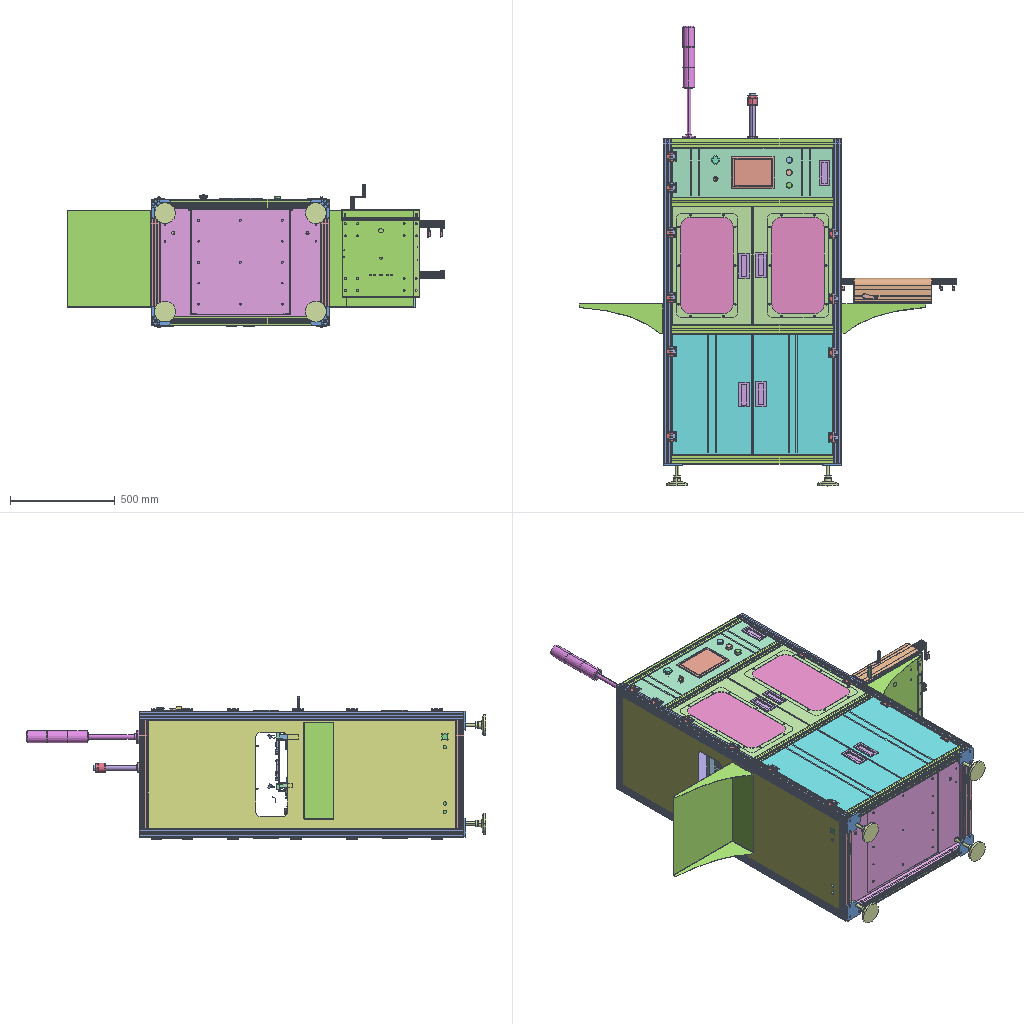Assembly | STEP file | 123 different items | 361 placed | box 1801 x 2194 x 686 mm
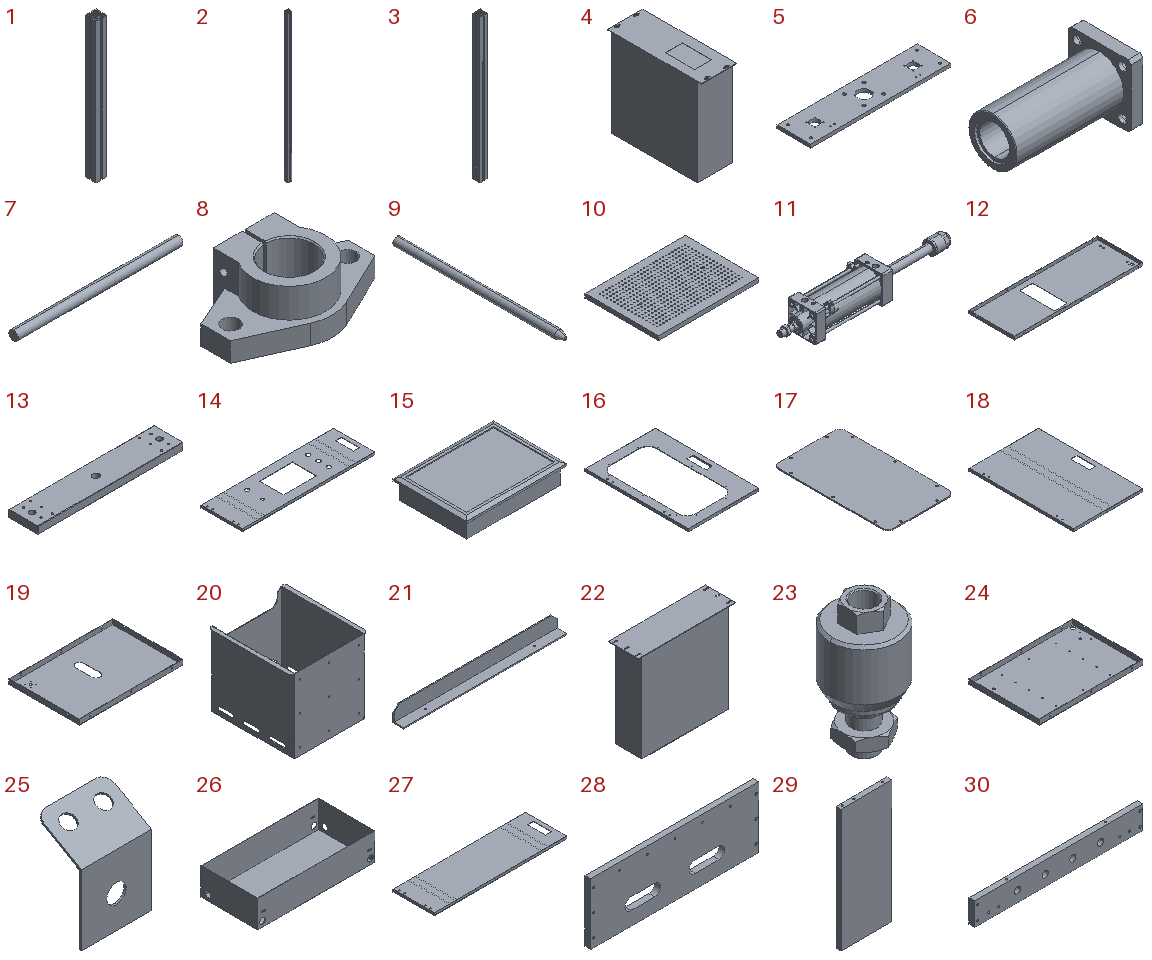Parts list (item | name | quantity | parent item | size | volume):
1 | Frame aluminum channel 3 | x9 | in FCT online single-layer test machine | 40 x 40 x 520 mm | 336590 mm3
2 | ICT frame aluminum channel 1 | x4 | in FCT online single-layer test machine | 40 x 40 x 1550 mm | 1003296 mm3
3 | Frame aluminum channel 2 | x8 | in FCT online single-layer test machine | 40 x 40 x 770 mm | 498412 mm3
4 | Industrial PC | x1 | in FCT online single-layer test machine | 180 x 480 x 450 mm | 35646453 mm3
5 | Hold-down fixture fixing plate | x1 | in FCT online single-layer test machine | 500 x 120 x 12 mm | 670055 mm3
6 | LMK20LUU  | x2 | in FCT online single-layer test machine | 80 x 42 x 42 mm | 44458 mm3
7 | Hold-down sync guide rod | x2 | in FCT online single-layer test machine | 350 x 20 x 20 mm | 109206 mm3
8 | SHF20 | x2 | in FCT online single-layer test machine | 60 x 36.276 x 20 mm | 15283 mm3
9 | Press rod | x4 | in FCT online single-layer test machine | 6 x 125 x 6 mm | 3458 mm3
10 | FCT press block | x1 | in FCT online single-layer test machine | 480 x 350 x 20 mm | 3170211 mm3
11 | SCJ_80x150_20_S_A_2_0020_ retract | x1 | in FCT online single-layer test machine | - | -
12 | ICT side seal plate | x2 | in FCT online single-layer test machine | 1468 x 518 x 38 mm | 1263222 mm3
13 | Hold-down fixture fixing plate | x1 | in FCT online single-layer test machine | 400 x 80 x 20 mm | 625122 mm3
14 | Front upper door | x1 | in FCT online single-layer test machine | 767 x 237 x 15 mm | 445389 mm3
15 | Xinje TH765 touch screen | x1 | in FCT online single-layer test machine | 204 x 150.5 x 44 mm | 1119032 mm3
16 | Middle door | x4 | in Door | 382.5 x 565 x 15 mm | 308904 mm3
17 | PVC sealing plate | x4 | in Door | 290 x 500 x 5 mm | 719804 mm3
18 | Bottom door | x4 | in FCT online single-layer test machine | 382.5 x 579 x 15 mm | 596109 mm3
19 | Top seal plate | x1 | in FCT online single-layer test machine | 768 x 518 x 38 mm | 719559 mm3
20 | Electrical cabinet box | x1 | in FCT online single-layer test machine | 520 x 560 x 500 mm | 2941429 mm3
21 | Electrical cabinet partition strip | x1 | in FCT online single-layer test machine | 450 x 30 x 40 mm | 89657 mm3
22 | FCT electrical control box | x1 | in FCT online single-layer test machine | 520 x 160 x 483 mm | 872599 mm3
23 | F-M20150F floating joint_HI | x1 | in FCT online single-layer test machine | 53 x 53 x 102 mm | 127493 mm3
24 | Bottom seal plate | x1 | in FCT online single-layer test machine | 768 x 518 x 38 mm | 730452 mm3
25 | Fiber fixing plate | x2 | in FCT online single-layer test machine, Conveyor test structure assembly | 20 x 13.29 x 27.5 mm | 382.645 mm3
26 | ICT test machine electrical box | x1 | in FCT online single-layer test machine | 515 x 250 x 120 mm | 459009 mm3
27 | Rear upper door | x1 | in FCT online single-layer test machine | 767 x 237 x 15 mm | 502024 mm3
28 | Rear side plate | x1 | in Test assembly | 425 x 15 x 155 mm | 907498 mm3
29 | Left-right side plate | x1 | in Test assembly | 155 x 15 x 375 mm | 868144 mm3
30 | Front side plate B | x1 | in Test assembly | 425 x 15 x 58 mm | 353146 mm3
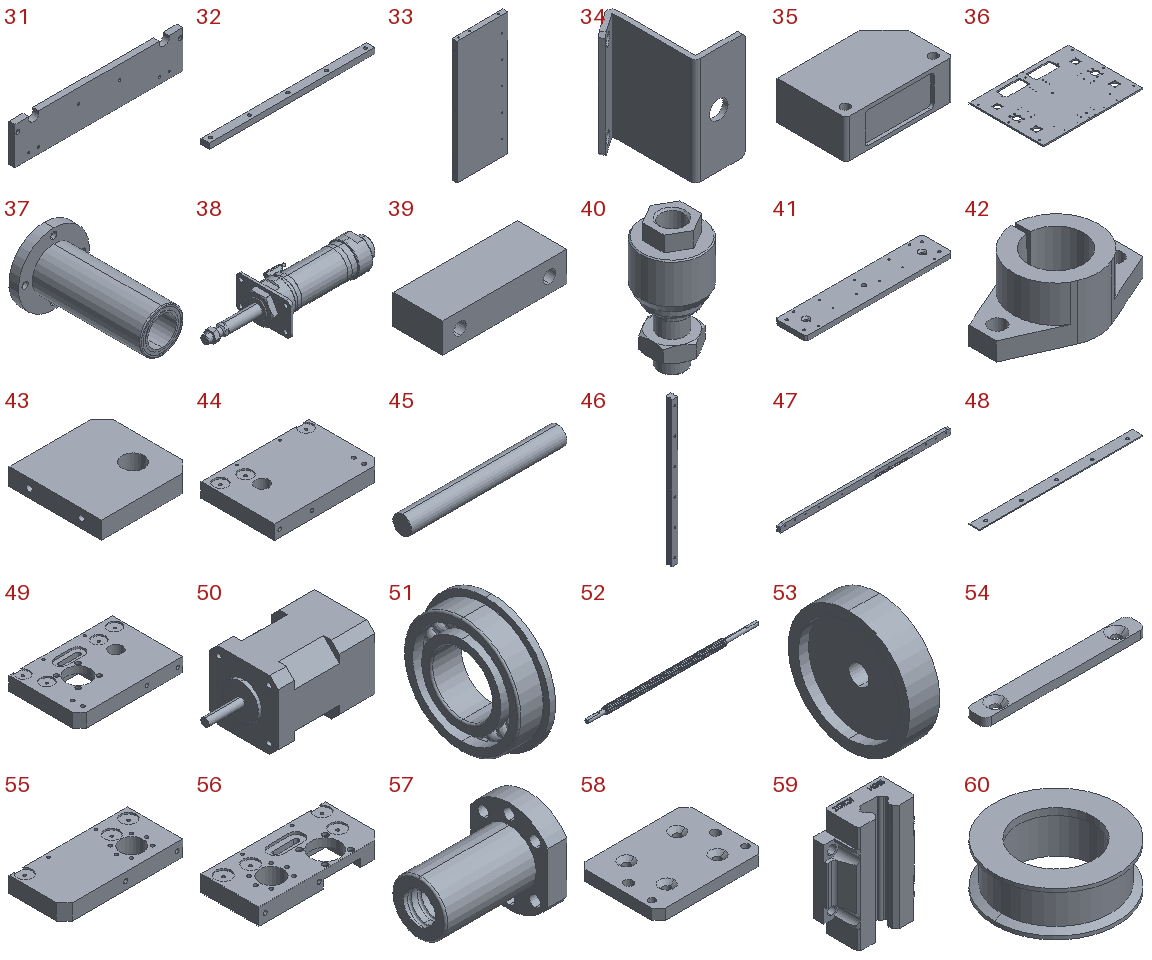31 | Front side plate A | x1 | in Test assembly | 425 x 15 x 95 mm | 590562 mm3
32 | Glass fixing plate | x4 | in Test assembly | 300 x 15 x 10 mm | 42251 mm3
33 | Left-right side plate A | x1 | in Test assembly | 155 x 15 x 375 mm | 868153 mm3
34 | Photoelectric switch mounting plate | x2 | in Photoelectric switch assembly | 22.414 x 26.5 x 32 mm | 2228 mm3
35 | CX421 | x2 | in Photoelectric switch assembly | 31.036 x 20.036 x 11.2 mm | 6433 mm3
36 | Platform plate | x1 | in Test mechanism assembly | 765 x 570 x 10 mm | 3949080 mm3
37 | LMF30LUU | x4 | in Test mechanism assembly | 74 x 123 x 74 mm | 132378 mm3
38 | MAL40x50-S-CM-FA-M-2 synchronous | x2 | in Test mechanism assembly | - | -
39 | Cylinder pad plate | x4 | in Test mechanism assembly | 50 x 20 x 12 mm | 11215 mm3
40 | F-M12125F floating joint | x2 | in Test mechanism assembly | 28 x 28 x 58 mm | 19289 mm3
41 | Width adjustment base | x2 | in Rail assembly | 380 x 80 x 12 mm | 356572 mm3
42 | SHF30 | x4 | in Rail assembly | 80 x 48 x 30 mm | 36862 mm3
43 | Lead screw rear fixing plate | x2 | in Rail assembly | 80 x 80 x 15 mm | 89638 mm3
44 | Front rail (left) | x1 | in Rail assembly | 150 x 102 x 20 mm | 295247 mm3
45 | Rail sync guide rod | x4 | in Rail assembly | 250 x 30 x 30 mm | 175961 mm3
46 | 15 guide rail | x2 | in Rail assembly | 15 x 15 x 330 mm | 60891 mm3
47 | Rail | x2 | in Rail assembly, Rear rail assembly | 840 x 15 x 30 mm | 357627 mm3
48 | Belt bracket plate | x2 | in Rail assembly, Rear rail assembly | 530 x 34 x 3 mm | 53588 mm3
49 | Front rail (right) | x1 | in Rail assembly | 150 x 102 x 20 mm | 257499 mm3
50 | Stepper motor CT2H420068-011 | x2 | in Rail assembly, Rear rail assembly | 84 x 42.3 x 42.3 mm | 101112 mm3
51 | miniature radial ball bearings gb_Rolling bearings FF61800  GB 7218-1995 | x4 | in Rail assembly | 5 x 21 x 21 mm | 818.239 mm3
52 | 1605 ball screw | x2 | in Rail assembly | 440 x 16 x 16 mm | 67458 mm3
53 | Handle | x2 | in Rail assembly | 25 x 60 x 60 mm | 35825 mm3
54 | Belt support strip | x4 | in Rail assembly, Rear rail assembly | 80 x 10 x 4 mm | 2948 mm3
55 | Rear rail (left) | x1 | in Rear rail assembly | 150 x 70 x 20 mm | 191088 mm3
56 | Rear rail (right) | x1 | in Rear rail assembly | 150 x 70 x 20 mm | 154483 mm3
57 | SHF1605 nut | x2 | in Rear rail assembly | 57 x 40 x 48 mm | 31691 mm3
58 | Slider connection plate | x2 | in Rear rail assembly | 80 x 60 x 8 mm | 35674 mm3
59 | HGW15CC slider | x2 | in Rear rail assembly | 47 x 19.7 x 61.7 mm | 35571 mm3
60 | 602-08-0005 | x16 | in 604 bearing assembly | 18 x 18 x 6.5 mm | 669.421 mm3
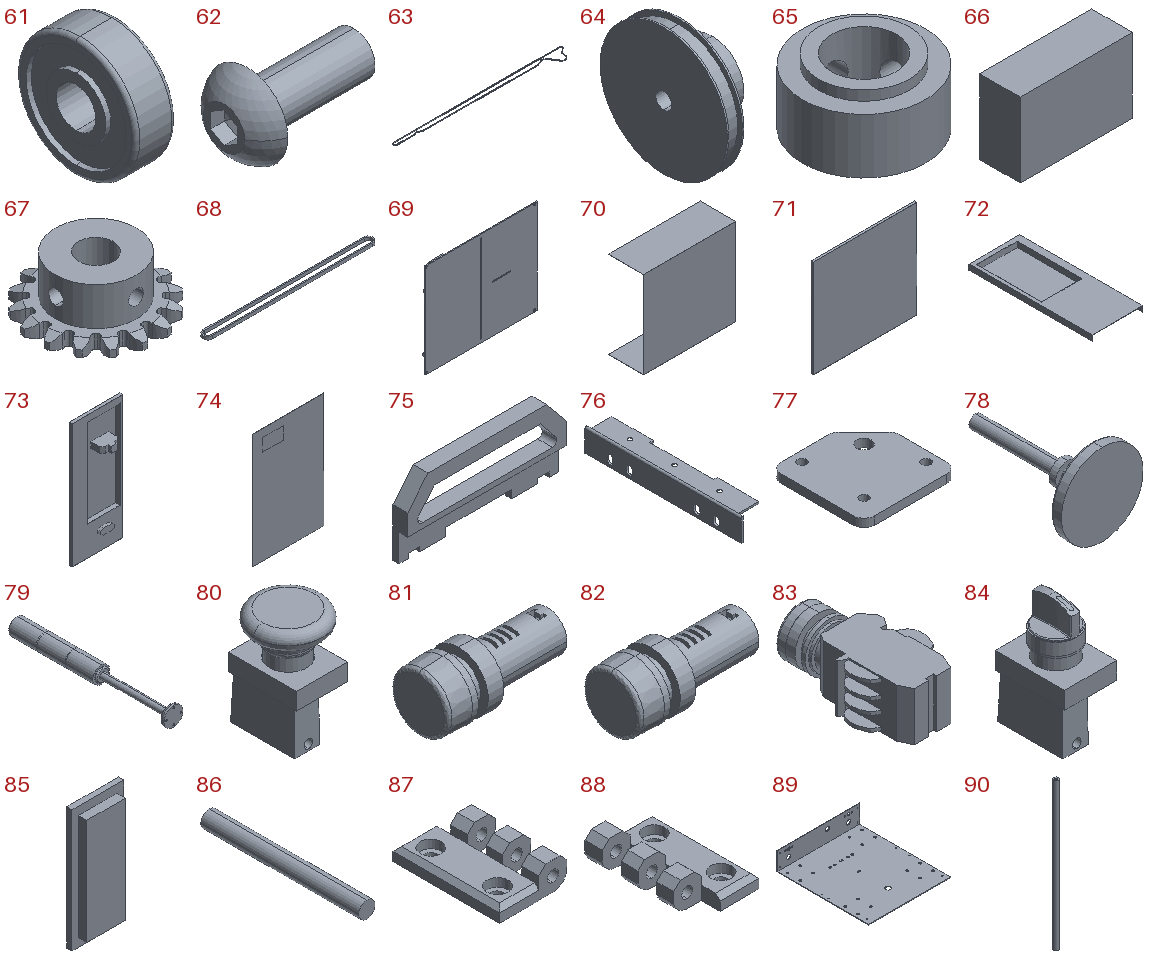61 | 604 bearing | x16 | in 604 bearing assembly | 4 x 12 x 12 mm | 349.308 mm3
62 | hexagon socket button head screws gb_GB_SOCKET_TYPE7 M4X10-N | x16 | in 604 bearing assembly | 12.2 x 7.6 x 7.6 mm | 185.741 mm3
63 | Belt | x2 | in Rear rail assembly, Rail assembly | 833 x 69.5 x 4 mm | 6996 mm3
64 | Belt drive pulley | x2 | in Rail assembly | 15.2 x 40 x 40 mm | 8508 mm3
65 | 602-03-0014 | x3 | in Rail assembly, Conveyor drive assembly | 19 x 19 x 10 mm | 1729 mm3
66 | Plate | x1 | in Conveyor test structure assembly | 416 x 170 x 276 mm | 18168400 mm3
67 | Sprocket 1/4in-10 | x2 | in Conveyor test structure assembly | 35.544 x 35.544 x 15 mm | 6436 mm3
68 | 1/4in chain | x1 | in Conveyor test structure assembly | 658 x 38 x 12 mm | 80620 mm3
69 | PCB board | x1 | in Conveyor test structure assembly | 250 x 17 x 210 mm | 172722 mm3
70 | Chassis side seal plate B_RR | x1 | in computer assembly_main_asm | 450 x 173 x 425 mm | 346050 mm3
71 | Chassis side seal plate A_RR | x1 | in computer assembly_main_asm | 452 x 10 x 427 mm | 208790 mm3
72 | Chassis front plate_RR | x1 | in computer assembly_main_asm | 177 x 427 x 20 mm | 104897 mm3
73 | Computer chassis rear plate_RR | x1 | in computer assembly_main_asm | 172 x 51 x 423 mm | 154052 mm3
74 | Computer chassis front-side small door RR | x1 | in computer assembly_main_asm | 140 x 1 x 225 mm | 31400 mm3
75 | Computer handle_RR | x1 | in Computer handle assembly RR ASM | 175 x 16 x 80 mm | 87445 mm3
76 | Rear computer plate rib part | x1 | in Computer handle assembly RR ASM | 25 x 176 x 26 mm | 15403 mm3
77 | 40 aluminum channel cup foot plate | x4 | in M16 cup foot assembly drawing | 90 x 90 x 8 mm | 58057 mm3
78 | M16 cup foot | x4 | in M16 cup foot assembly drawing | 100 x 155 x 100 mm | 165556 mm3
79 | Alarm light | x1 | in FCT online single-layer test machine | 65 x 539.374 x 65 mm | 871558 mm3
80 | PX950 (w)2) | x1 | in FCT online single-layer test machine | 40 x 40 x 60 mm | 29605 mm3
81 | 22 green indicator light | x1 | in FCT online single-layer test machine | 65 x 30 x 30 mm | 34522 mm3
82 | 22 red indicator light | x1 | in FCT online single-layer test machine | 65 x 30 x 30 mm | 34522 mm3
83 | 22 self-locking illuminated pushbutton _LA42PSD-O black | x1 | in FCT online single-layer test machine | 44.081 x 82 x 30 mm | 65737 mm3
84 | Power switch | x1 | in FCT online single-layer test machine | 30 x 40 x 65 mm | 19689 mm3
85 | Aluminum pull handle | x10 | in FCT online single-layer test machine | 49.768 x 13 x 118.027 mm | 32136 mm3
86 | HHPSJ6_B_shaft | x20 | in HHPSJ648X48_HHPSJ6-B | 5 x 48 x 5 mm | 942.478 mm3
87 | HHPSJ6_B_l | x20 | in HHPSJ648X48_HHPSJ6-B | 30.3 x 48 x 12.8 mm | 7045 mm3
88 | HHPSJ6_B_r | x20 | in HHPSJ648X48_HHPSJ6-B | 30.1 x 48 x 12.8 mm | 7008 mm3
89 | 601-01-0067 | x1 | in Conveyor drive assembly | 370 x 415 x 85 mm | 542185 mm3
90 | 602-12-0049 | x2 | in Conveyor drive assembly | 12 x 12 x 370 mm | 41119 mm3
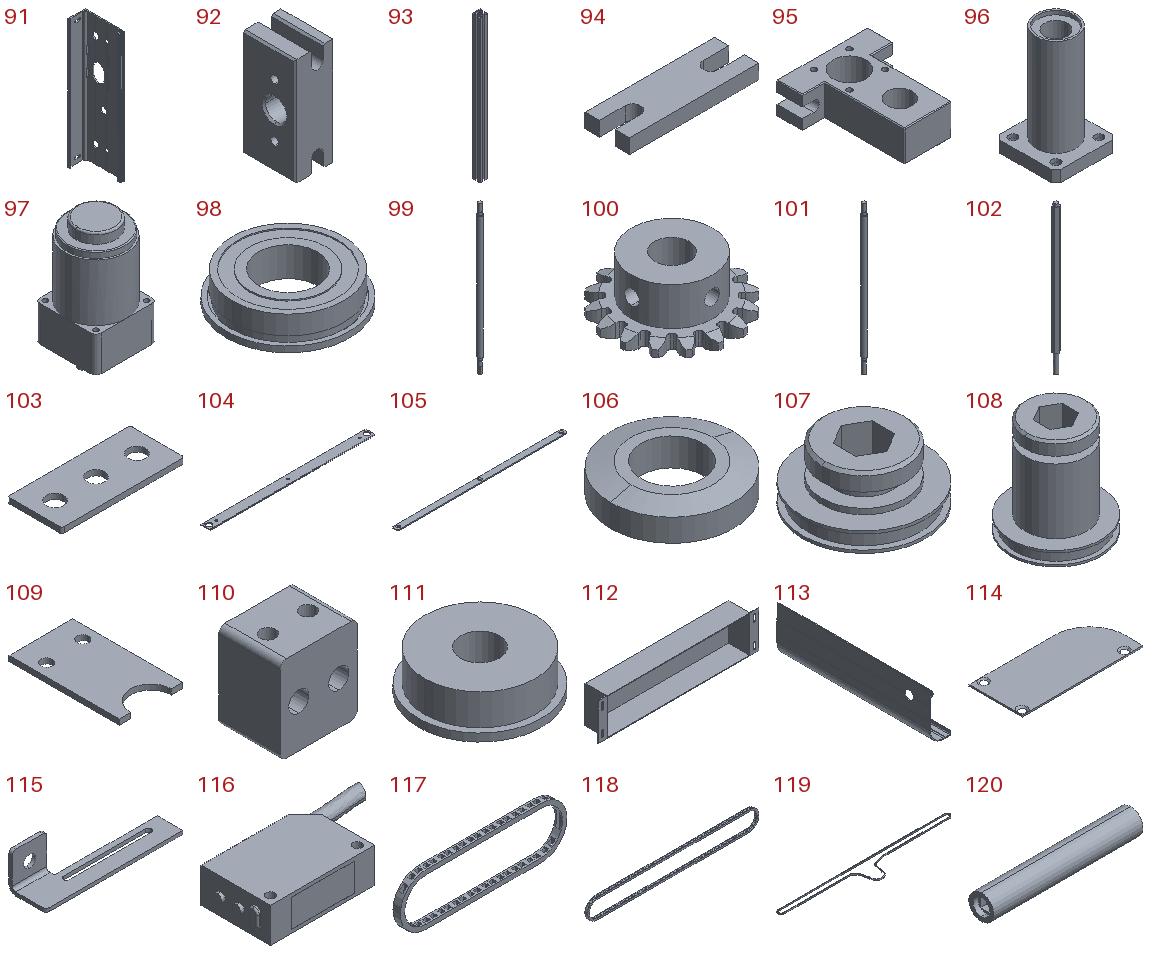91 | 601-12-0009 | x1 | in Conveyor drive assembly | 50.06 x 115 x 370 mm | 200376 mm3
92 | 602-03-0012 | x2 | in Conveyor drive assembly | 22 x 29 x 60 mm | 31178 mm3
93 | 602-13-0039 | x2 | in Conveyor drive assembly | 30 x 30 x 550 mm | 186584 mm3
94 | 601-07-0071 | x4 | in Conveyor drive assembly | 58 x 20 x 6.5 mm | 6243 mm3
95 | 602-03-0011 | x2 | in Conveyor drive assembly | 58 x 66.996 x 20 mm | 35380 mm3
96 | 202-02-0006 | x2 | in Conveyor drive assembly | 32 x 32 x 57 mm | 15769 mm3
97 | 101-03-0011 | x1 | in Conveyor drive assembly | 70 x 70 x 156.5 mm | 487470 mm3
98 | 202-01-0017 | x6 | in Conveyor drive assembly | 21 x 21 x 5 mm | 1023 mm3
99 | 602-09-0048 | x1 | in Conveyor drive assembly | 14 x 14 x 425 mm | 59315 mm3
100 | 103-01-0008 | x4 | in Conveyor drive assembly | 35.544 x 35.544 x 15 mm | 6436 mm3
101 | 602-09-0047 | x1 | in Conveyor drive assembly | 14 x 14 x 425 mm | 59824 mm3
102 | 602-12-0050 | x1 | in Conveyor drive assembly | 14 x 16.166 x 398 mm | 62104 mm3
103 | 601-07-0010 | x4 | in Conveyor drive assembly | 45 x 20 x 2 mm | 1599 mm3
104 | 602-01-0036 | x2 | in Conveyor drive assembly | 550 x 30 x 3 mm | 47601 mm3
105 | 602-06-0016 | x2 | in Conveyor drive assembly | 498 x 16 x 3 mm | 23447 mm3
106 | 601-07-0094 | x8 | in Conveyor drive assembly | 12 x 12 x 2.7 mm | 212.267 mm3
107 | 103-01-0007 | x1 | in Conveyor drive assembly | 44 x 44 x 20 mm | 13109 mm3
108 | 103-01-0006 | x1 | in Conveyor drive assembly | 44 x 44 x 48 mm | 28816 mm3
109 | 601-07-0070 | x1 | in Conveyor drive assembly | 36 x 62 x 3 mm | 5874 mm3
110 | 601-07-0069 | x4 | in Conveyor drive assembly | 25 x 20 x 28 mm | 10875 mm3
111 | 202-01-0015 | x8 | in Conveyor drive assembly | 19 x 19 x 6 mm | 1260 mm3
112 | 601-01-0066 | x1 | in Conveyor drive assembly | 370 x 50 x 85 mm | 106591 mm3
113 | 601-10-0092 | x1 | in Conveyor drive assembly | 52 x 370 x 118 mm | 126535 mm3
114 | 601-01-0001 | x2 | in Conveyor drive assembly | 118 x 52 x 1.5 mm | 8586 mm3
115 | 601-07-0012 | x3 | in Conveyor drive assembly | 80 x 21.644 x 21.644 mm | 2963 mm3
116 | 501-04-0011 | x3 | in Conveyor drive assembly | 47.887 x 22.217 x 10 mm | 6035 mm3
117 | 1/4in chain | x1 | in Conveyor drive assembly | 112.8 x 5 x 35 mm | 2655 mm3
118 | 1/4in long chain | x1 | in Conveyor drive assembly | 305 x 5 x 35 mm | 6649 mm3
119 | Anti-static belt | x2 | in Conveyor drive assembly | 544 x 77.5 x 4 mm | 7074 mm3
120 | Handle B | x1 | in Adjusting handle assembly drawing | 90 x 15 x 15 mm | 11283 mm3
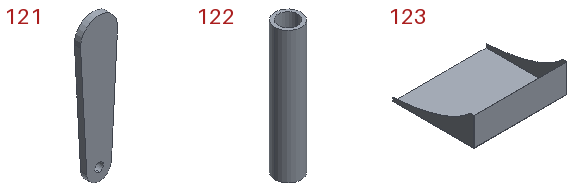121 | Handwheel sub-plate | x1 | in Adjusting handle assembly drawing | 18 x 3 x 70 mm | 2988 mm3
122 | Handle A | x1 | in Adjusting handle assembly drawing | 12 x 12 x 60 mm | 5168 mm3
123 | Conveyor belt fixing plate | x2 | in FCT online single-layer test machine | 463 x 401.5 x 141.5 mm | 444630 mm3
Placements (level | parent | child | x y z in mm | rotation matrix by rows), first 284 of 416 lines:
1 | FCT online single-layer test machine | Frame aluminum channel 3 | -244.865 -95.172 -260.0 | 1 0 0 0 1 0 0 0 1
1 | FCT online single-layer test machine | Frame aluminum channel 3 | -244.865 1414.828 -260.0 | 1 0 0 0 1 0 0 0 1
1 | FCT online single-layer test machine | Frame aluminum channel 3 | 565.135 -95.172 -260.0 | 1 0 0 0 1 0 0 0 1
1 | FCT online single-layer test machine | Frame aluminum channel 3 | 565.135 1414.828 -260.0 | 1 0 0 0 1 0 0 0 1
1 | FCT online single-layer test machine | ICT frame aluminum channel 1 | 78.951 1528.341 49.698 | 0 -1 0 0 0 -1 1 0 -0
1 | FCT online single-layer test machine | ICT frame aluminum channel 1 | 78.951 1528.341 -510.302 | 0 -1 0 0 0 -1 1 0 -0
1 | FCT online single-layer test machine | ICT frame aluminum channel 1 | 888.951 1528.341 49.698 | 0 -1 0 0 0 -1 1 0 -0
1 | FCT online single-layer test machine | ICT frame aluminum channel 1 | 888.951 1528.341 -510.302 | 0 -1 0 0 0 -1 1 0 -0
1 | FCT online single-layer test machine | Frame aluminum channel 2 | 775.437 228.644 186.486 | 0 0 -1 -1 0 0 0 1 -0
1 | FCT online single-layer test machine | Frame aluminum channel 2 | 775.437 1738.644 186.486 | 0 0 -1 -1 0 0 0 1 -0
1 | FCT online single-layer test machine | Frame aluminum channel 2 | 775.437 228.644 -373.514 | 0 0 -1 -1 0 0 0 1 -0
1 | FCT online single-layer test machine | Frame aluminum channel 2 | 775.437 1738.644 -373.514 | 0 0 -1 -1 0 0 0 1 -0
1 | FCT online single-layer test machine | Frame aluminum channel 2 | 775.437 850.644 -373.514 | 0 0 -1 -1 0 0 0 1 -0
1 | FCT online single-layer test machine | Frame aluminum channel 2 | 775.437 850.644 186.486 | 0 0 -1 -1 0 0 0 1 -0
1 | FCT online single-layer test machine | Industrial PC | 556.225 141.358 -195.5 | 0 1 0 -1 0 0 0 0 1
1 | FCT online single-layer test machine | Frame aluminum channel 2 | 775.437 1458.644 -373.514 | 0 0 -1 -1 0 0 0 1 -0
1 | FCT online single-layer test machine | Frame aluminum channel 2 | 775.437 1458.644 186.486 | 0 0 -1 -1 0 0 0 1 -0
1 | FCT online single-layer test machine | Hold-down fixture fixing plate | 351.646 1248.341 3.611 | 1 0 0 0 0 1 0 -1 -0
1 | FCT online single-layer test machine | LMK20LUU  | 599.959 1188.341 40.386 | 0 0 -1 1 0 0 0 -1 -0
1 | FCT online single-layer test machine | LMK20LUU  | 206.472 1188.341 65.943 | 0 1 0 1 0 0 0 0 -1
1 | FCT online single-layer test machine | Hold-down sync guide rod | 538.837 1473.341 59.154 | 0 -0.3118 0.9501 -1 0 0 0 -0.9501 -0.3118
1 | FCT online single-layer test machine | Hold-down sync guide rod | 177.926 1473.341 23.081 | 0 0.6503 0.7597 -1 0 0 0 -0.7597 0.6503
1 | FCT online single-layer test machine | SHF20 | 215.437 1123.341 31.421 | 0 1 0 0 0 1 1 0 -0
1 | FCT online single-layer test machine | SHF20 | 565.437 1123.341 31.421 | 0 1 0 0 0 1 1 0 0
1 | FCT online single-layer test machine | Press rod | 177.747 972.775 134.652 | 0.9994 0 -0.03387 0 1 0 0.03387 0 0.9994
1 | FCT online single-layer test machine | FCT press block | 360.815 1103.341 163.016 | 1 0 0 0 0 -1 0 1 0
1 | FCT online single-layer test machine | Frame aluminum channel 3 | 522.635 526.828 -260.0 | 1 0 0 0 1 0 0 0 1
1 | FCT online single-layer test machine | Frame aluminum channel 3 | -202.365 526.828 -260.0 | 1 0 0 0 1 0 0 0 1
1 | FCT online single-layer test machine | SCJ_80x150_20_S_A_2_0020_ retract | 390.437 1260.341 31.421 | 0 -1 0 1 0 0 0 0 1
1 | FCT online single-layer test machine | ICT side seal plate | 815.437 1285.27 221.826 | 0 0 -1 -1 0 0 0 1 -0
1 | FCT online single-layer test machine | ICT side seal plate | -34.563 1285.27 -221.826 | 0 0 1 -1 0 0 0 -1 0
1 | FCT online single-layer test machine | Hold-down fixture fixing plate | 252.948 1123.341 40.477 | 1 0 0 0 0 -1 0 1 0
1 | FCT online single-layer test machine | Frame aluminum channel 3 | -69.865 1134.828 -260.0 | 1 0 0 0 1 0 0 0 1
1 | FCT online single-layer test machine | Frame aluminum channel 3 | 390.135 1134.828 -260.0 | 1 0 0 0 1 0 0 0 1
1 | FCT online single-layer test machine | Front upper door | 390.437 1367.841 285.0 | 1 0 0 0 1 0 0 0 1
1 | FCT online single-layer test machine | Xinje TH765 touch screen | 340.266 1410.195 263.0 | 1 0 0 0 1 0 0 0 1
1 | FCT online single-layer test machine | Door | 266.866 931.967 292.5 | 1 0 0 0 1 0 0 0 1
2 | Door | Middle door | -206.971 212.363 -7.5 | 1 0 0 0 1 0 0 0 1
2 | Door | PVC sealing plate | -68.679 101.908 0.5 | 1 0 0 0 1 0 0 0 1
1 | FCT online single-layer test machine | Door | 514.008 916.716 292.5 | -1 0 0 0 -1 0 0 0 1
2 | Door | Middle door | -206.971 212.363 -7.5 | 1 0 0 0 1 0 0 0 1
2 | Door | PVC sealing plate | -68.679 101.908 0.5 | 1 0 0 0 1 0 0 0 1
1 | FCT online single-layer test machine | Door | 514.008 931.967 -292.5 | -1 0 0 0 1 0 0 0 -1
2 | Door | Middle door | -206.971 212.363 -7.5 | 1 0 0 0 1 0 0 0 1
2 | Door | PVC sealing plate | -68.679 101.908 0.5 | 1 0 0 0 1 0 0 0 1
1 | FCT online single-layer test machine | Door | 266.866 916.716 -292.5 | 1 0 0 0 -1 0 0 0 -1
2 | Door | Middle door | -206.971 212.363 -7.5 | 1 0 0 0 1 0 0 0 1
2 | Door | PVC sealing plate | -68.679 101.908 0.5 | 1 0 0 0 1 0 0 0 1
1 | FCT online single-layer test machine | Bottom door | 59.895 536.33 285.0 | 1 0 0 0 1 0 0 0 1
1 | FCT online single-layer test machine | Bottom door | 720.979 82.353 285.0 | -1 0 0 0 -1 0 0 0 1
1 | FCT online single-layer test machine | Bottom door | 59.895 82.353 -285.0 | 1 0 0 0 -1 0 0 0 -1
1 | FCT online single-layer test machine | Bottom door | 720.979 536.33 -285.0 | -1 0 0 0 1 0 0 0 -1
1 | FCT online single-layer test machine | Top seal plate | 156.589 1528.341 219.749 | 1 0 0 0 0 -1 0 1 0
1 | FCT online single-layer test machine | Frame aluminum channel 3 | 160.135 526.828 -260.0 | 1 0 0 0 1 0 0 0 1
1 | FCT online single-layer test machine | Electrical cabinet box | 390.437 -1.659 -248.5 | 1 0 0 0 1 0 0 0 1
1 | FCT online single-layer test machine | Electrical cabinet partition strip | 208.19 388.275 225.0 | 0 0 1 0 1 0 -1 0 0
1 | FCT online single-layer test machine | FCT electrical control box | 196.303 550.321 251.5 | 1 0 0 0 1 0 0 0 1
1 | FCT online single-layer test machine | F-M20150F floating joint_HI | 390.437 1103.341 31.421 | 0.9763 -0.2164 0 0 0 1 -0.2164 -0.9763 -0
1 | FCT online single-layer test machine | Bottom seal plate | 156.589 18.341 219.749 | 1 0 0 0 0 -1 0 1 -0
1 | FCT online single-layer test machine | Fiber fixing plate | 485.205 852.205 -130.528 | 1 0 0 0 1 0 0 0 1
1 | FCT online single-layer test machine | ICT test machine electrical box | 186.232 1470.816 120.0 | 1 0 0 0 1 0 0 0 1
1 | FCT online single-layer test machine | Rear upper door | 389.937 1368.841 -285.0 | -1 0 0 0 1 0 0 0 -1
1 | FCT online single-layer test machine | Test assembly | 390.437 650.341 -198.288 | 1 0 0 0 0 1 0 -1 0
2 | Test assembly | Rear side plate | -0.0 -0.0 -0.0 | 1 0 0 0 1 0 0 0 1
2 | Test assembly | Left-right side plate | 176.898 -7.5 99.753 | 0 -1 0 0 0 -1 1 0 0
2 | Test assembly | Front side plate B | -0.0 -390.0 58.0 | 1 0 0 0 -1 0 0 0 -1
2 | Test assembly | Front side plate A | -0.0 -390.0 60.0 | 1 0 0 0 1 0 0 0 1
2 | Test assembly | Glass fixing plate | -0.0 -17.5 137.5 | -1 0 0 0 0 1 0 1 0
2 | Test assembly | Glass fixing plate | -187.5 -195.0 137.5 | 0 0 -1 -1 0 0 0 1 0
2 | Test assembly | Glass fixing plate | 187.5 -195.0 137.5 | 0 0 1 1 0 0 0 1 0
2 | Test assembly | Glass fixing plate | -0.0 -372.5 137.5 | 1 0 0 0 0 -1 0 1 0
2 | Test assembly | Left-right side plate A | -233.102 -7.5 99.753 | 0 -1 0 0 0 -1 1 0 0
1 | FCT online single-layer test machine | Photoelectric switch assembly | 436.437 873.341 -59.306 | 0 0 1 0 1 0 -1 0 0
2 | Photoelectric switch assembly | Photoelectric switch mounting plate | -0.0 -0.0 -0.0 | 1 0 0 0 1 0 0 0 1
2 | Photoelectric switch assembly | CX421 | -2.434 31.963 -0.0 | 0 0.8192 -0.5736 0 0.5736 0.8192 1 0 -0
1 | FCT online single-layer test machine | Press rod | 552.747 972.775 134.652 | 0.9994 0 -0.03387 0 1 0 0.03387 0 0.9994
1 | FCT online single-layer test machine | Press rod | 552.747 972.775 -69.348 | 0.9994 0 -0.03387 0 1 0 0.03387 0 0.9994
1 | FCT online single-layer test machine | Press rod | 177.747 972.775 -69.348 | 0.9994 0 -0.03387 0 1 0 0.03387 0 0.9994
1 | FCT online single-layer test machine | Conveyor test structure assembly | 708.772 640.341 236.677 | 1 0 0 0 0 1 0 -1 0
2 | Conveyor test structure assembly | Test mechanism assembly | -0.0 -0.0 -0.0 | 1 0 0 0 1 0 0 0 1
3 | Test mechanism assembly | Platform plate | -0.0 -0.0 -0.0 | 1 0 0 0 1 0 0 0 1
3 | Test mechanism assembly | LMF30LUU | -576.73 423.129 -103.0 | 0.7071 0 0.7071 0.7071 0 -0.7071 0 1 0
3 | Test mechanism assembly | LMF30LUU | -581.034 44.222 -103.0 | 0.7071 0 -0.7071 -0.7071 0 -0.7071 0 1 0
3 | Test mechanism assembly | LMF30LUU | -59.941 48.526 -103.0 | -0.7071 0 -0.7071 -0.7071 0 0.7071 0 1 -0
3 | Test mechanism assembly | LMF30LUU | 23.27 423.129 -103.0 | 0.7071 0 0.7071 0.7071 0 -0.7071 0 1 0
3 | Test mechanism assembly | MAL40x50-S-CM-FA-M-2 synchronous | -612.004 253.785 26.0 | 0 0 -1 0 -1 0 -1 0 -0
3 | Test mechanism assembly | MAL40x50-S-CM-FA-M-2 synchronous | -24.667 217.87 16.0 | 0 0 1 0 1 0 -1 0 0
3 | Test mechanism assembly | Cylinder pad plate | 101.417 276.827 -37.174 | 1 0 0 0 0 -1 0 1 0
3 | Test mechanism assembly | Cylinder pad plate | 101.417 194.827 7.174 | 1 0 0 0 0 1 0 -1 -0
3 | Test mechanism assembly | Cylinder pad plate | -498.583 276.827 -37.174 | 1 0 0 0 0 -1 0 1 0
3 | Test mechanism assembly | Cylinder pad plate | -498.583 206.827 -37.174 | 1 0 0 0 0 -1 0 1 0
3 | Test mechanism assembly | F-M12125F floating joint | -618.335 235.827 121.5 | -0.05752 -0.9983 0 -0.9983 0.05752 0 0 0 -1
3 | Test mechanism assembly | F-M12125F floating joint | -18.335 235.827 111.5 | -0.05752 -0.9983 0 -0.9983 0.05752 0 0 0 -1
2 | Conveyor test structure assembly | Rail assembly | -608.449 364.978 104.0 | 0 1 0 -1 0 0 0 0 1
3 | Rail assembly | Width adjustment base | -0.0 -0.0 -0.0 | 1 0 0 0 1 0 0 0 1
3 | Rail assembly | SHF30 | -157428.927 24736.852 -0.0 | 0 -1 0 -1 0 0 0 0 -1
3 | Rail assembly | SHF30 | 157687.227 -24756.625 -0.0 | 0 1 0 1 0 0 0 0 -1
3 | Rail assembly | Lead screw rear fixing plate | -35.85 -0.8307 133.907 | 0 0 -1 0 1 0 1 0 -0
3 | Rail assembly | Front rail (left) | 316.65 184.035 64.0 | 0 0 -1 -1 0 0 0 1 0
3 | Rail assembly | Rail sync guide rod | 27.683 -16.127 -250.0 | 0 -0.02122 -0.9998 0 0.9998 -0.02122 1 0 0
3 | Rail assembly | Rail sync guide rod | 327.683 -16.127 -250.0 | 0 -0.02122 -0.9998 0 0.9998 -0.02122 1 0 0
3 | Rail assembly | 15 guide rail | 219.15 -19.887 27.0 | 0 0 -1 -1 0 0 0 1 0
3 | Rail assembly | Rail | 326.65 498.98 114.0 | 0 0 -1 -1 0 0 0 1 0
3 | Rail assembly | Belt bracket plate | 292.65 310.676 114.0 | 0 -1 0 -1 0 0 0 0 -1
3 | Rail assembly | Front rail (right) | 316.65 874.035 64.0 | 0 0 -1 -1 0 0 0 1 0
3 | Rail assembly | Stepper motor CT2H420068-011 | 306.65 648.609 41.262 | 1 0 0 0 1 0 0 0 1
3 | Rail assembly | miniature radial ball bearings gb_Rolling bearings FF61800  GB 7218-1995 | 298.15 600.113 69.0 | -1 0 0 0 0.08787 -0.9961 0 -0.9961 -0.08787
3 | Rail assembly | 1605 ball screw | 340.65 600.113 69.0 | -1 0 0 0 -0.2556 -0.9668 0 -0.9668 0.2556
3 | Rail assembly | Handle | 340.65 600.113 69.0 | -1 0 0 0 0.5461 -0.8377 0 -0.8377 -0.5461
3 | Rail assembly | Width adjustment base | -0.0 580.227 12.0 | 1 0 0 0 -1 0 0 0 -1
3 | Rail assembly | Lead screw rear fixing plate | -50.85 581.057 133.907 | 0 0 1 0 -1 0 1 0 -0
3 | Rail assembly | 15 guide rail | 219.15 600.113 27.0 | 0 0 -1 -1 0 0 0 1 0
3 | Rail assembly | miniature radial ball bearings gb_Rolling bearings FF61800  GB 7218-1995 | 298.15 -19.887 69.0 | -1 0 0 0 0.08787 -0.9961 0 -0.9961 -0.08787
3 | Rail assembly | 1605 ball screw | 340.65 -19.887 69.0 | -1 0 0 0 0.8521 -0.5234 0 -0.5234 -0.8521
3 | Rail assembly | SHF30 | -157428.927 25336.852 0.0 | 0 -1 0 -1 0 0 0 0 -1
3 | Rail assembly | SHF30 | 157687.227 -24156.625 0.0 | 0 1 0 1 0 0 0 0 -1
3 | Rail assembly | Rail sync guide rod | 11.248 553.18 -250.0 | 0 0.649 -0.7608 0 0.7608 0.649 1 0 0
3 | Rail assembly | Rail sync guide rod | 312.884 554.668 -250.0 | 0 0.6139 -0.7894 0 0.7894 0.6139 1 0 0
3 | Rail assembly | Belt support strip | 296.65 -143.855 95.932 | 0 0 -1 -1 0 0 0 1 0
3 | Rail assembly | Belt support strip | 296.65 546.145 95.932 | 0 0 -1 -1 0 0 0 1 0
3 | Rail assembly | Rear rail assembly | 53.994 81.246 114.0 | 0 0 1 1 0 0 0 1 0
4 | Rear rail assembly | Rail | 0.0 0.0 -0.0 | 1 0 0 0 1 0 0 0 1
4 | Rear rail assembly | Rear rail (left) | -375.054 -50.0 10.0 | 1 0 0 0 1 0 0 0 1
4 | Rear rail assembly | Rear rail (right) | 314.946 -50.0 10.0 | 1 0 0 0 1 0 0 0 1
4 | Rear rail assembly | Belt bracket plate | 188.304 0.0 34.0 | 1 0 0 0 0 -1 0 1 0
4 | Rear rail assembly | SHF1605 nut | -101.133 -45.0 -0.0 | 0 0 1 0 1 0 -1 0 0
4 | Rear rail assembly | SHF1605 nut | 518.867 -45.0 0.0 | 0 0 1 0 1 0 -1 0 0
4 | Rear rail assembly | Stepper motor CT2H420068-011 | 556.131 -61.506 20.0 | 0 0 1 0 1 0 -1 0 0
4 | Rear rail assembly | Belt support strip | 642.835 -18.068 30.0 | 1 0 0 0 1 0 0 0 1
4 | Rear rail assembly | Belt support strip | -47.165 -18.068 30.0 | 1 0 0 0 1 0 0 0 1
4 | Rear rail assembly | Slider connection plate | -13.826 -78.0 28.005 | 1 0 0 0 0 1 0 -1 -0
4 | Rear rail assembly | Slider connection plate | 606.174 -78.0 28.005 | 1 0 0 0 0 1 0 -1 -0
4 | Rear rail assembly | HGW15CC slider | -101.133 -87.0 20.0 | 1 0 0 0 1 0 0 0 1
4 | Rear rail assembly | HGW15CC slider | 518.867 -87.0 20.0 | 1 0 0 0 1 0 0 0 1
4 | Rear rail assembly | 604 bearing assembly | 616.867 -8.0 30.0 | 0.9503 -0.3114 0 0.3114 0.9503 0 0 0 1
5 | 604 bearing assembly | 602-08-0005 | -0.0 -0.0 -0.0 | 1 0 0 0 1 0 0 0 1
5 | 604 bearing assembly | 604 bearing | 0.0 -0.0 3.25 | 0 0 -1 0 1 0 1 0 -0
5 | 604 bearing assembly | hexagon socket button head screws gb_GB_SOCKET_TYPE7 M4X10-N | 0.0 0.0 7.45 | 0 0 1 0 1 0 -1 0 0
4 | Rear rail assembly | 604 bearing assembly | 608.867 -35.0 30.0 | 0.9815 -0.1917 0 0.1917 0.9815 0 0 0 1
5 | 604 bearing assembly | 602-08-0005 | -0.0 -0.0 -0.0 | 1 0 0 0 1 0 0 0 1
5 | 604 bearing assembly | 604 bearing | 0.0 -0.0 3.25 | 0 0 -1 0 1 0 1 0 -0
5 | 604 bearing assembly | hexagon socket button head screws gb_GB_SOCKET_TYPE7 M4X10-N | 0.0 0.0 7.45 | 0 0 1 0 1 0 -1 0 0
4 | Rear rail assembly | 604 bearing assembly | 518.867 -20.0 30.0 | 0.9815 -0.1917 0 0.1917 0.9815 0 0 0 1
5 | 604 bearing assembly | 602-08-0005 | -0.0 -0.0 -0.0 | 1 0 0 0 1 0 0 0 1
5 | 604 bearing assembly | 604 bearing | 0.0 -0.0 3.25 | 0 0 -1 0 1 0 1 0 -0
5 | 604 bearing assembly | hexagon socket button head screws gb_GB_SOCKET_TYPE7 M4X10-N | 0.0 0.0 7.45 | 0 0 1 0 1 0 -1 0 0
4 | Rear rail assembly | 604 bearing assembly | 490.867 -15.0 30.0 | 0.9815 -0.1917 0 0.1917 0.9815 0 0 0 1
5 | 604 bearing assembly | 602-08-0005 | -0.0 -0.0 -0.0 | 1 0 0 0 1 0 0 0 1
5 | 604 bearing assembly | 604 bearing | 0.0 -0.0 3.25 | 0 0 -1 0 1 0 1 0 -0
5 | 604 bearing assembly | hexagon socket button head screws gb_GB_SOCKET_TYPE7 M4X10-N | 0.0 0.0 7.45 | 0 0 1 0 1 0 -1 0 0
4 | Rear rail assembly | 604 bearing assembly | 548.867 -20.0 30.0 | 0.9815 -0.1917 0 0.1917 0.9815 0 0 0 1
5 | 604 bearing assembly | 602-08-0005 | -0.0 -0.0 -0.0 | 1 0 0 0 1 0 0 0 1
5 | 604 bearing assembly | 604 bearing | 0.0 -0.0 3.25 | 0 0 -1 0 1 0 1 0 -0
5 | 604 bearing assembly | hexagon socket button head screws gb_GB_SOCKET_TYPE7 M4X10-N | 0.0 0.0 7.45 | 0 0 1 0 1 0 -1 0 0
4 | Rear rail assembly | 604 bearing assembly | -73.133 -13.0 30.0 | -0.001174 1 0 -1 -0.001174 0 0 0 1
5 | 604 bearing assembly | 602-08-0005 | -0.0 -0.0 -0.0 | 1 0 0 0 1 0 0 0 1
5 | 604 bearing assembly | 604 bearing | 0.0 -0.0 3.25 | 0 0 -1 0 1 0 1 0 -0
5 | 604 bearing assembly | hexagon socket button head screws gb_GB_SOCKET_TYPE7 M4X10-N | 0.0 0.0 7.45 | 0 0 1 0 1 0 -1 0 0
4 | Rear rail assembly | 604 bearing assembly | -101.133 -20.0 30.0 | -0.9591 0.2832 0 -0.2832 -0.9591 0 0 0 1
5 | 604 bearing assembly | 602-08-0005 | -0.0 -0.0 -0.0 | 1 0 0 0 1 0 0 0 1
5 | 604 bearing assembly | 604 bearing | 0.0 -0.0 3.25 | 0 0 -1 0 1 0 1 0 -0
5 | 604 bearing assembly | hexagon socket button head screws gb_GB_SOCKET_TYPE7 M4X10-N | 0.0 0.0 7.45 | 0 0 1 0 1 0 -1 0 0
4 | Rear rail assembly | 604 bearing assembly | -199.133 -8.0 30.0 | -0.6746 -0.7382 0 0.7382 -0.6746 0 0 0 1
5 | 604 bearing assembly | 602-08-0005 | -0.0 -0.0 -0.0 | 1 0 0 0 1 0 0 0 1
5 | 604 bearing assembly | 604 bearing | 0.0 -0.0 3.25 | 0 0 -1 0 1 0 1 0 -0
5 | 604 bearing assembly | hexagon socket button head screws gb_GB_SOCKET_TYPE7 M4X10-N | 0.0 0.0 7.45 | 0 0 1 0 1 0 -1 0 0
4 | Rear rail assembly | Belt | 208.864 -8.005 31.0 | 1 0 0 0 1 0 0 0 1
3 | Rail assembly | Belt drive pulley | 68524.382 -6211.035 -27679.932 | 1 0 0 0 0.2404 -0.9707 0 0.9707 0.2404
3 | Rail assembly | Belt drive pulley | -68143.738 -14856.947 -23939.318 | -1 0 0 0 0.5429 0.8398 0 0.8398 -0.5429
3 | Rail assembly | 604 bearing assembly | 296.65 698.113 106.0 | 0 0 -1 -0.1071 0.9942 0 0.9942 0.1071 0
4 | 604 bearing assembly | 602-08-0005 | -0.0 -0.0 -0.0 | 1 0 0 0 1 0 0 0 1
4 | 604 bearing assembly | 604 bearing | 0.0 -0.0 3.25 | 0 0 -1 0 1 0 1 0 -0
4 | 604 bearing assembly | hexagon socket button head screws gb_GB_SOCKET_TYPE7 M4X10-N | 0.0 0.0 7.45 | 0 0 1 0 1 0 -1 0 0
3 | Rail assembly | 604 bearing assembly | 296.65 690.113 79.0 | 0 0 -1 -0.1071 0.9942 0 0.9942 0.1071 0
4 | 604 bearing assembly | 602-08-0005 | -0.0 -0.0 -0.0 | 1 0 0 0 1 0 0 0 1
4 | 604 bearing assembly | 604 bearing | 0.0 -0.0 3.25 | 0 0 -1 0 1 0 1 0 -0
4 | 604 bearing assembly | hexagon socket button head screws gb_GB_SOCKET_TYPE7 M4X10-N | 0.0 0.0 7.45 | 0 0 1 0 1 0 -1 0 0
3 | Rail assembly | 604 bearing assembly | 296.65 572.113 99.0 | 0 0 -1 -0.5602 0.8284 0 0.8284 0.5602 0
4 | 604 bearing assembly | 602-08-0005 | -0.0 -0.0 -0.0 | 1 0 0 0 1 0 0 0 1
4 | 604 bearing assembly | 604 bearing | 0.0 -0.0 3.25 | 0 0 -1 0 1 0 1 0 -0
4 | 604 bearing assembly | hexagon socket button head screws gb_GB_SOCKET_TYPE7 M4X10-N | 0.0 0.0 7.45 | 0 0 1 0 1 0 -1 0 0
3 | Rail assembly | 604 bearing assembly | 296.65 600.113 94.0 | 0 0 -1 -0.1071 0.9942 0 0.9942 0.1071 0
4 | 604 bearing assembly | 602-08-0005 | -0.0 -0.0 -0.0 | 1 0 0 0 1 0 0 0 1
4 | 604 bearing assembly | 604 bearing | 0.0 -0.0 3.25 | 0 0 -1 0 1 0 1 0 -0
4 | 604 bearing assembly | hexagon socket button head screws gb_GB_SOCKET_TYPE7 M4X10-N | 0.0 0.0 7.45 | 0 0 1 0 1 0 -1 0 0
3 | Rail assembly | 604 bearing assembly | 296.65 630.113 94.0 | 0 0 -1 -0.1071 0.9942 0 0.9942 0.1071 0
4 | 604 bearing assembly | 602-08-0005 | -0.0 -0.0 -0.0 | 1 0 0 0 1 0 0 0 1
4 | 604 bearing assembly | 604 bearing | 0.0 -0.0 3.25 | 0 0 -1 0 1 0 1 0 -0
4 | 604 bearing assembly | hexagon socket button head screws gb_GB_SOCKET_TYPE7 M4X10-N | 0.0 0.0 7.45 | 0 0 1 0 1 0 -1 0 0
3 | Rail assembly | 604 bearing assembly | 296.65 8.113 99.0 | 0 0 -1 -0.1071 0.9942 0 0.9942 0.1071 0
4 | 604 bearing assembly | 602-08-0005 | -0.0 -0.0 -0.0 | 1 0 0 0 1 0 0 0 1
4 | 604 bearing assembly | 604 bearing | 0.0 -0.0 3.25 | 0 0 -1 0 1 0 1 0 -0
4 | 604 bearing assembly | hexagon socket button head screws gb_GB_SOCKET_TYPE7 M4X10-N | 0.0 0.0 7.45 | 0 0 1 0 1 0 -1 0 0
3 | Rail assembly | 604 bearing assembly | 296.65 -117.887 106.0 | 0 0 -1 -0.1071 0.9942 0 0.9942 0.1071 0
4 | 604 bearing assembly | 602-08-0005 | -0.0 -0.0 -0.0 | 1 0 0 0 1 0 0 0 1
4 | 604 bearing assembly | 604 bearing | 0.0 -0.0 3.25 | 0 0 -1 0 1 0 1 0 -0
4 | 604 bearing assembly | hexagon socket button head screws gb_GB_SOCKET_TYPE7 M4X10-N | 0.0 0.0 7.45 | 0 0 1 0 1 0 -1 0 0
3 | Rail assembly | 604 bearing assembly | 296.65 -19.887 92.0 | 0 0 -1 -0.1071 0.9942 0 0.9942 0.1071 0
4 | 604 bearing assembly | 602-08-0005 | -0.0 -0.0 -0.0 | 1 0 0 0 1 0 0 0 1
4 | 604 bearing assembly | 604 bearing | 0.0 -0.0 3.25 | 0 0 -1 0 1 0 1 0 -0
4 | 604 bearing assembly | hexagon socket button head screws gb_GB_SOCKET_TYPE7 M4X10-N | 0.0 0.0 7.45 | 0 0 1 0 1 0 -1 0 0
3 | Rail assembly | miniature radial ball bearings gb_Rolling bearings FF61800  GB 7218-1995 | -37.35 -19.887 69.0 | 1 0 0 0 -0.2911 -0.9567 0 0.9567 -0.2911
3 | Rail assembly | miniature radial ball bearings gb_Rolling bearings FF61800  GB 7218-1995 | -37.35 600.113 69.0 | 1 0 0 0 -0.4723 -0.8814 0 0.8814 -0.4723
3 | Rail assembly | 602-03-0014 | -24.85 600.113 69.0 | 0 0 -1 0.9713 0.2378 0 0.2378 -0.9713 -0
3 | Rail assembly | 602-03-0014 | -24.85 -19.887 69.0 | 0 0 -1 0.6882 -0.7255 0 -0.7255 -0.6882 -0
3 | Rail assembly | Belt | 291.15 290.111 105.995 | 0 0 1 1 0 0 0 1 0
3 | Rail assembly | Handle | 340.65 -19.887 69.0 | -1 0 0 0 0.5461 -0.8377 0 -0.8377 -0.5461
2 | Conveyor test structure assembly | Plate | -348.844 40.327 118.087 | 1 0 0 0 0 -1 0 1 0
2 | Conveyor test structure assembly | Fiber fixing plate | -378.776 42.317 206.864 | -1 0 0 0 0 1 0 1 0
2 | Conveyor test structure assembly | Photoelectric switch assembly | -409.35 53.327 233.0 | 0 0 -1 -1 0 0 0 1 0
3 | Photoelectric switch assembly | Photoelectric switch mounting plate | -0.0 -0.0 -0.0 | 1 0 0 0 1 0 0 0 1
3 | Photoelectric switch assembly | CX421 | -2.434 31.963 -0.0 | 0 0.8192 -0.5736 0 0.5736 0.8192 1 0 -0
2 | Conveyor test structure assembly | Sprocket 1/4in-10 | -628.335 421.827 173.0 | 0.985 0.1726 0 0 0 1 0.1726 -0.985 0
2 | Conveyor test structure assembly | Sprocket 1/4in-10 | -8.335 421.827 173.0 | 0.985 0.1726 0 0 0 1 0.1726 -0.985 0
2 | Conveyor test structure assembly | 1/4in chain | -318.335 423.827 173.0 | 1 0 0 0 0 -1 0 1 0
2 | Conveyor test structure assembly | PCB board | -318.333 173.327 218.495 | 1 0 0 0 0 -1 0 1 0
1 | FCT online single-layer test machine | computer assembly_main_asm | 368.437 211.341 -18.5 | 0 0 -1 0 1 0 1 0 -0
2 | computer assembly_main_asm | Chassis side seal plate B_RR | -0.0 -0.0 -0.0 | 1 0 0 0 1 0 0 0 1
2 | computer assembly_main_asm | Chassis side seal plate A_RR | -0.0 174.0 -0.0 | 1 0 0 0 -1 0 0 0 -1
2 | computer assembly_main_asm | Chassis front plate_RR | 227.0 86.5 -0.0 | 0 0 1 -1 0 0 0 -1 0
2 | computer assembly_main_asm | Computer chassis rear plate_RR | -225.0 87.0 -0.0 | 0 1 0 -1 0 0 0 0 1
2 | computer assembly_main_asm | Computer chassis front-side small door RR | 227.0 93.0 -86.0 | 0 -1 0 1 0 0 0 0 1
2 | computer assembly_main_asm | Computer handle assembly RR ASM | 197.0 86.5 -211.0 | 0 0 1 -1 0 0 0 -1 0
3 | Computer handle assembly RR ASM | Computer handle_RR | -0.0 -0.0 -0.0 | 1 0 0 0 1 0 0 0 1
3 | Computer handle assembly RR ASM | Rear computer plate rib part | -0.0 6.0 30.0 | 0 1 0 0 0 -1 -1 0 0
1 | FCT online single-layer test machine | M16 cup foot assembly drawing | 10.437 -29.659 255.0 | 1 0 0 0 0 1 0 -1 -0
2 | M16 cup foot assembly drawing | 40 aluminum channel cup foot plate | -0.0 -0.0 -0.0 | 1 0 0 0 1 0 0 0 1
2 | M16 cup foot assembly drawing | M16 cup foot | 20.0 20.0 -62.0 | 1 0 0 0 0 -1 0 1 -0
1 | FCT online single-layer test machine | M16 cup foot assembly drawing | 770.437 -29.659 -255.0 | -1 0 0 0 0 1 0 1 0
2 | M16 cup foot assembly drawing | 40 aluminum channel cup foot plate | -0.0 -0.0 -0.0 | 1 0 0 0 1 0 0 0 1
2 | M16 cup foot assembly drawing | M16 cup foot | 20.0 20.0 -62.0 | 1 0 0 0 0 -1 0 1 -0
1 | FCT online single-layer test machine | M16 cup foot assembly drawing | 770.437 -29.659 255.0 | 0 -1 0 0 0 1 -1 0 0
2 | M16 cup foot assembly drawing | 40 aluminum channel cup foot plate | -0.0 -0.0 -0.0 | 1 0 0 0 1 0 0 0 1
2 | M16 cup foot assembly drawing | M16 cup foot | 20.0 20.0 -62.0 | 1 0 0 0 0 -1 0 1 -0
1 | FCT online single-layer test machine | M16 cup foot assembly drawing | 10.437 -29.659 -255.0 | 0 1 0 0 0 1 1 0 0
2 | M16 cup foot assembly drawing | 40 aluminum channel cup foot plate | -0.0 -0.0 -0.0 | 1 0 0 0 1 0 0 0 1
2 | M16 cup foot assembly drawing | M16 cup foot | 20.0 20.0 -62.0 | 1 0 0 0 0 -1 0 1 -0
1 | FCT online single-layer test machine | Alarm light | 86.437 1921.716 179.0 | 1 0 0 0 1 0 0 0 1
1 | FCT online single-layer test machine | PX950 (w)2) | 214.437 1427.841 285.0 | 1 0 0 0 1 0 0 0 1
1 | FCT online single-layer test machine | 22 green indicator light | 566.437 1367.841 277.109 | 0 0 1 0 1 0 -1 0 0
1 | FCT online single-layer test machine | 22 red indicator light | 566.437 1307.841 277.109 | 0 0 1 0 1 0 -1 0 0
1 | FCT online single-layer test machine | 22 self-locking illuminated pushbutton _LA42PSD-O black | 566.437 1427.841 312.0 | 1 0 0 0 0 -1 0 1 0
1 | FCT online single-layer test machine | Power switch | 214.437 1337.841 285.0 | 1 0 0 0 1 0 0 0 1
1 | FCT online single-layer test machine | Aluminum pull handle | 734.437 1366.841 292.0 | 1 0 0 0 0 -1 0 1 0
1 | FCT online single-layer test machine | HHPSJ648X48_HHPSJ6-B | 2.937 1445.841 306.5 | 1 0 0 0 1 0 0 0 1
2 | HHPSJ648X48_HHPSJ6-B | HHPSJ6_B_shaft | -0.0 -0.0 -0.0 | 1 0 0 0 1 0 0 0 1
2 | HHPSJ648X48_HHPSJ6-B | HHPSJ6_B_l | -0.0 -24.0 -6.5 | 1 0 0 0 1 0 0 0 1
2 | HHPSJ648X48_HHPSJ6-B | HHPSJ6_B_r | -0.0 -24.0 -6.5 | 1 0 0 0 1 0 0 0 1
1 | FCT online single-layer test machine | HHPSJ648X48_HHPSJ6-B | 2.937 1295.841 306.5 | 1 0 0 0 1 0 0 0 1
2 | HHPSJ648X48_HHPSJ6-B | HHPSJ6_B_shaft | -0.0 -0.0 -0.0 | 1 0 0 0 1 0 0 0 1
2 | HHPSJ648X48_HHPSJ6-B | HHPSJ6_B_l | -0.0 -24.0 -6.5 | 1 0 0 0 1 0 0 0 1
2 | HHPSJ648X48_HHPSJ6-B | HHPSJ6_B_r | -0.0 -24.0 -6.5 | 1 0 0 0 1 0 0 0 1
1 | FCT online single-layer test machine | HHPSJ648X48_HHPSJ6-B | 2.937 1082.341 306.5 | 1 0 0 0 1 0 0 0 1
2 | HHPSJ648X48_HHPSJ6-B | HHPSJ6_B_shaft | -0.0 -0.0 -0.0 | 1 0 0 0 1 0 0 0 1
2 | HHPSJ648X48_HHPSJ6-B | HHPSJ6_B_l | -0.0 -24.0 -6.5 | 1 0 0 0 1 0 0 0 1
2 | HHPSJ648X48_HHPSJ6-B | HHPSJ6_B_r | -0.0 -24.0 -6.5 | 1 0 0 0 1 0 0 0 1
1 | FCT online single-layer test machine | HHPSJ648X48_HHPSJ6-B | 2.937 772.341 306.5 | 1 0 0 0 1 0 0 0 1
2 | HHPSJ648X48_HHPSJ6-B | HHPSJ6_B_shaft | -0.0 -0.0 -0.0 | 1 0 0 0 1 0 0 0 1
2 | HHPSJ648X48_HHPSJ6-B | HHPSJ6_B_l | -0.0 -24.0 -6.5 | 1 0 0 0 1 0 0 0 1
2 | HHPSJ648X48_HHPSJ6-B | HHPSJ6_B_r | -0.0 -24.0 -6.5 | 1 0 0 0 1 0 0 0 1
1 | FCT online single-layer test machine | HHPSJ648X48_HHPSJ6-B | 777.937 766.341 306.5 | 1 0 0 0 1 0 0 0 1
2 | HHPSJ648X48_HHPSJ6-B | HHPSJ6_B_shaft | -0.0 -0.0 -0.0 | 1 0 0 0 1 0 0 0 1
2 | HHPSJ648X48_HHPSJ6-B | HHPSJ6_B_l | -0.0 -24.0 -6.5 | 1 0 0 0 1 0 0 0 1
2 | HHPSJ648X48_HHPSJ6-B | HHPSJ6_B_r | -0.0 -24.0 -6.5 | 1 0 0 0 1 0 0 0 1
1 | FCT online single-layer test machine | HHPSJ648X48_HHPSJ6-B | 777.937 1076.341 306.5 | 1 0 0 0 1 0 0 0 1
2 | HHPSJ648X48_HHPSJ6-B | HHPSJ6_B_shaft | -0.0 -0.0 -0.0 | 1 0 0 0 1 0 0 0 1
2 | HHPSJ648X48_HHPSJ6-B | HHPSJ6_B_l | -0.0 -24.0 -6.5 | 1 0 0 0 1 0 0 0 1
2 | HHPSJ648X48_HHPSJ6-B | HHPSJ6_B_r | -0.0 -24.0 -6.5 | 1 0 0 0 1 0 0 0 1
1 | FCT online single-layer test machine | HHPSJ648X48_HHPSJ6-B | 2.937 514.341 306.5 | 1 0 0 0 1 0 0 0 1
2 | HHPSJ648X48_HHPSJ6-B | HHPSJ6_B_shaft | -0.0 -0.0 -0.0 | 1 0 0 0 1 0 0 0 1
2 | HHPSJ648X48_HHPSJ6-B | HHPSJ6_B_l | -0.0 -24.0 -6.5 | 1 0 0 0 1 0 0 0 1
2 | HHPSJ648X48_HHPSJ6-B | HHPSJ6_B_r | -0.0 -24.0 -6.5 | 1 0 0 0 1 0 0 0 1
1 | FCT online single-layer test machine | HHPSJ648X48_HHPSJ6-B | 2.937 110.341 306.5 | 1 0 0 0 1 0 0 0 1
2 | HHPSJ648X48_HHPSJ6-B | HHPSJ6_B_shaft | -0.0 -0.0 -0.0 | 1 0 0 0 1 0 0 0 1
2 | HHPSJ648X48_HHPSJ6-B | HHPSJ6_B_l | -0.0 -24.0 -6.5 | 1 0 0 0 1 0 0 0 1
2 | HHPSJ648X48_HHPSJ6-B | HHPSJ6_B_r | -0.0 -24.0 -6.5 | 1 0 0 0 1 0 0 0 1
1 | FCT online single-layer test machine | HHPSJ648X48_HHPSJ6-B | 777.937 104.341 306.5 | 1 0 0 0 1 0 0 0 1
2 | HHPSJ648X48_HHPSJ6-B | HHPSJ6_B_shaft | -0.0 -0.0 -0.0 | 1 0 0 0 1 0 0 0 1
2 | HHPSJ648X48_HHPSJ6-B | HHPSJ6_B_l | -0.0 -24.0 -6.5 | 1 0 0 0 1 0 0 0 1
2 | HHPSJ648X48_HHPSJ6-B | HHPSJ6_B_r | -0.0 -24.0 -6.5 | 1 0 0 0 1 0 0 0 1
1 | FCT online single-layer test machine | HHPSJ648X48_HHPSJ6-B | 777.937 508.341 306.5 | 1 0 0 0 1 0 0 0 1
2 | HHPSJ648X48_HHPSJ6-B | HHPSJ6_B_shaft | -0.0 -0.0 -0.0 | 1 0 0 0 1 0 0 0 1
2 | HHPSJ648X48_HHPSJ6-B | HHPSJ6_B_l | -0.0 -24.0 -6.5 | 1 0 0 0 1 0 0 0 1
2 | HHPSJ648X48_HHPSJ6-B | HHPSJ6_B_r | -0.0 -24.0 -6.5 | 1 0 0 0 1 0 0 0 1